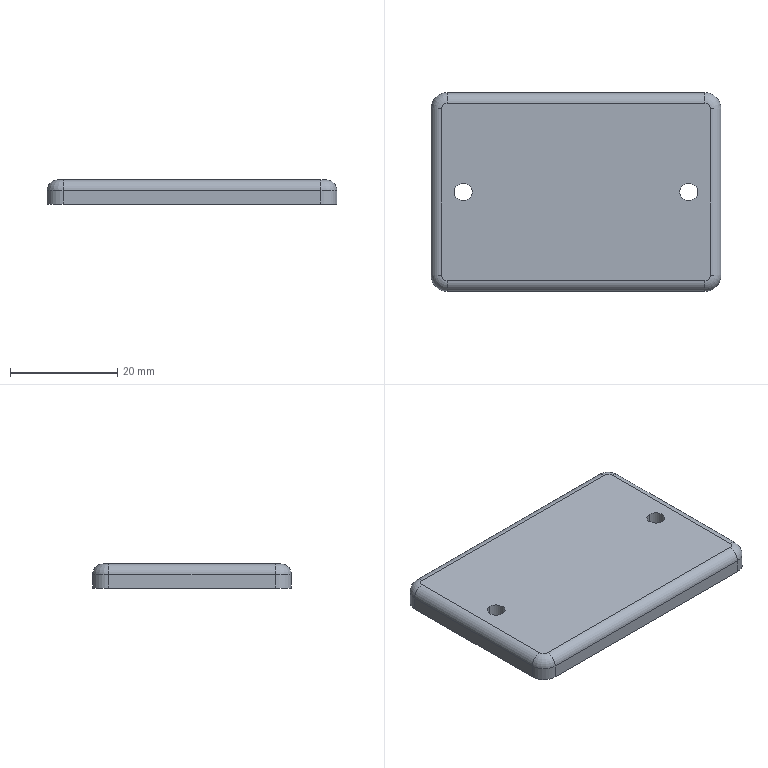Part | SolidWorks | features BaseBody 1 | 1 solid | 35 faces | box 54 x 37 x 4.5 mm | volume 8135 mm3 | cylinder 18 | plane 13 | torus 4 | commonest cylinder face diameters 11.3 x6 3.3 x4 4 x4 6 x4
STEP:
#1=CARTESIAN_POINT('',(-30.5,5.65,26.5));
#2=VERTEX_POINT('',#1);
#3=CARTESIAN_POINT('',(-30.5,5.65,26.));
#4=VERTEX_POINT('',#3);
#5=CARTESIAN_POINT('',(-30.5,5.65,31.5));
#6=DIRECTION('',(0.,0.,-1.));
#7=VECTOR('',#6,1000.);
#8=LINE('',#5,#7);
#9=EDGE_CURVE('',#2,#4,#8,.T.);
#10=ORIENTED_EDGE('',*,*,#9,.F.);
#11=CARTESIAN_POINT('',(-28.5,5.284,26.5));
#12=VERTEX_POINT('',#11);
#13=CARTESIAN_POINT('',(-30.5,0.,26.5));
#14=DIRECTION('',(0.,0.,1.));
#15=DIRECTION('',(0.,1.,0.));
#16=AXIS2_PLACEMENT_3D('',#13,#14,#15);
#17=CIRCLE('',#16,5.65);
#18=EDGE_CURVE('',#12,#2,#17,.T.);
#19=ORIENTED_EDGE('',*,*,#18,.F.);
#20=CARTESIAN_POINT('',(-28.5,5.284,26.));
#21=VERTEX_POINT('',#20);
#22=CARTESIAN_POINT('',(-28.5,5.284,31.5));
#23=DIRECTION('',(0.,0.,1.));
#24=VECTOR('',#23,1000.);
#25=LINE('',#22,#24);
#26=EDGE_CURVE('',#21,#12,#25,.T.);
#27=ORIENTED_EDGE('',*,*,#26,.F.);
#28=CARTESIAN_POINT('',(-30.5,0.,26.));
#29=DIRECTION('',(0.,0.,1.));
#30=DIRECTION('',(0.,1.,0.));
#31=AXIS2_PLACEMENT_3D('',#28,#29,#30);
#32=CIRCLE('',#31,5.65);
#33=EDGE_CURVE('',#21,#4,#32,.T.);
#34=ORIENTED_EDGE('',*,*,#33,.T.);
#35=EDGE_LOOP('',(#10,#19,#27,#34));
#36=FACE_OUTER_BOUND('',#35,.T.);
#37=CARTESIAN_POINT('',(-30.5,0.,31.5));
#38=DIRECTION('',(0.,0.,-1.));
#39=DIRECTION('',(0.,1.,0.));
#40=AXIS2_PLACEMENT_3D('',#37,#38,#39);
#41=CYLINDRICAL_SURFACE('',#40,5.65);
#42=ADVANCED_FACE('',(#36),#41,.T.);
#43=CARTESIAN_POINT('',(-72.5,-5.65,26.5));
#44=VERTEX_POINT('',#43);
#45=CARTESIAN_POINT('',(-72.5,-5.65,26.));
#46=VERTEX_POINT('',#45);
#47=CARTESIAN_POINT('',(-72.5,-5.65,31.5));
#48=DIRECTION('',(0.,0.,-1.));
#49=VECTOR('',#48,1000.);
#50=LINE('',#47,#49);
#51=EDGE_CURVE('',#44,#46,#50,.T.);
#52=ORIENTED_EDGE('',*,*,#51,.F.);
#53=CARTESIAN_POINT('',(-74.5,-5.284,26.5));
#54=VERTEX_POINT('',#53);
#55=CARTESIAN_POINT('',(-72.5,0.,26.5));
#56=DIRECTION('',(0.,0.,-1.));
#57=DIRECTION('',(0.,1.,0.));
#58=AXIS2_PLACEMENT_3D('',#55,#56,#57);
#59=CIRCLE('',#58,5.65);
#60=EDGE_CURVE('',#44,#54,#59,.T.);
#61=ORIENTED_EDGE('',*,*,#60,.T.);
#62=CARTESIAN_POINT('',(-74.5,-5.284,26.));
#63=VERTEX_POINT('',#62);
#64=CARTESIAN_POINT('',(-74.5,-5.284,31.5));
#65=DIRECTION('',(0.,0.,-1.));
#66=VECTOR('',#65,1000.);
#67=LINE('',#64,#66);
#68=EDGE_CURVE('',#54,#63,#67,.T.);
#69=ORIENTED_EDGE('',*,*,#68,.T.);
#70=CARTESIAN_POINT('',(-72.5,0.,26.));
#71=DIRECTION('',(0.,0.,-1.));
#72=DIRECTION('',(0.,1.,0.));
#73=AXIS2_PLACEMENT_3D('',#70,#71,#72);
#74=CIRCLE('',#73,5.65);
#75=EDGE_CURVE('',#46,#63,#74,.T.);
#76=ORIENTED_EDGE('',*,*,#75,.F.);
#77=EDGE_LOOP('',(#52,#61,#69,#76));
#78=FACE_OUTER_BOUND('',#77,.T.);
#79=CARTESIAN_POINT('',(-72.5,0.,31.5));
#80=DIRECTION('',(0.,0.,-1.));
#81=DIRECTION('',(0.,1.,0.));
#82=AXIS2_PLACEMENT_3D('',#79,#80,#81);
#83=CYLINDRICAL_SURFACE('',#82,5.65);
#84=ADVANCED_FACE('',(#78),#83,.T.);
#85=CARTESIAN_POINT('',(-28.5,-14.5,26.5));
#86=VERTEX_POINT('',#85);
#87=CARTESIAN_POINT('',(-28.5,-14.5,26.));
#88=VERTEX_POINT('',#87);
#89=CARTESIAN_POINT('',(-28.5,-14.5,29.5));
#90=DIRECTION('',(0.,0.,-1.));
#91=VECTOR('',#90,1000.);
#92=LINE('',#89,#91);
#93=EDGE_CURVE('',#86,#88,#92,.T.);
#94=ORIENTED_EDGE('',*,*,#93,.T.);
#95=CARTESIAN_POINT('',(-74.5,-14.5,26.));
#96=VERTEX_POINT('',#95);
#97=CARTESIAN_POINT('',(-75.5,-14.5,26.));
#98=DIRECTION('',(-1.,0.,0.));
#99=VECTOR('',#98,1000.);
#100=LINE('',#97,#99);
#101=EDGE_CURVE('',#88,#96,#100,.T.);
#102=ORIENTED_EDGE('',*,*,#101,.T.);
#103=CARTESIAN_POINT('',(-74.5,-14.5,26.5));
#104=VERTEX_POINT('',#103);
#105=CARTESIAN_POINT('',(-74.5,-14.5,29.5));
#106=DIRECTION('',(0.,0.,-1.));
#107=VECTOR('',#106,1000.);
#108=LINE('',#105,#107);
#109=EDGE_CURVE('',#104,#96,#108,.T.);
#110=ORIENTED_EDGE('',*,*,#109,.F.);
#111=CARTESIAN_POINT('',(-27.5,-14.5,26.5));
#112=DIRECTION('',(1.,0.,0.));
#113=VECTOR('',#112,1000.);
#114=LINE('',#111,#113);
#115=EDGE_CURVE('',#104,#86,#114,.T.);
#116=ORIENTED_EDGE('',*,*,#115,.T.);
#117=EDGE_LOOP('',(#94,#102,#110,#116));
#118=FACE_OUTER_BOUND('',#117,.T.);
#119=CARTESIAN_POINT('',(-27.5,-14.5,29.5));
#120=DIRECTION('',(0.,-1.,0.));
#121=DIRECTION('',(0.,0.,-1.));
#122=AXIS2_PLACEMENT_3D('',#119,#120,#121);
#123=PLANE('',#122);
#124=ADVANCED_FACE('',(#118),#123,.F.);
#125=CARTESIAN_POINT('',(-28.5,-5.284,26.));
#126=VERTEX_POINT('',#125);
#127=CARTESIAN_POINT('',(-28.5,15.5,26.));
#128=DIRECTION('',(0.,-1.,0.));
#129=VECTOR('',#128,1000.);
#130=LINE('',#127,#129);
#131=EDGE_CURVE('',#126,#88,#130,.T.);
#132=ORIENTED_EDGE('',*,*,#131,.T.);
#133=ORIENTED_EDGE('',*,*,#93,.F.);
#134=CARTESIAN_POINT('',(-28.5,-5.284,26.5));
#135=VERTEX_POINT('',#134);
#136=CARTESIAN_POINT('',(-28.5,15.5,26.5));
#137=DIRECTION('',(0.,-1.,0.));
#138=VECTOR('',#137,1000.);
#139=LINE('',#136,#138);
#140=EDGE_CURVE('',#135,#86,#139,.T.);
#141=ORIENTED_EDGE('',*,*,#140,.F.);
#142=CARTESIAN_POINT('',(-28.5,-5.284,31.5));
#143=DIRECTION('',(0.,0.,-1.));
#144=VECTOR('',#143,1000.);
#145=LINE('',#142,#144);
#146=EDGE_CURVE('',#135,#126,#145,.T.);
#147=ORIENTED_EDGE('',*,*,#146,.T.);
#148=EDGE_LOOP('',(#132,#133,#141,#147));
#149=FACE_OUTER_BOUND('',#148,.T.);
#150=CARTESIAN_POINT('',(-28.5,15.5,29.5));
#151=DIRECTION('',(1.,0.,0.));
#152=DIRECTION('',(0.,1.,0.));
#153=AXIS2_PLACEMENT_3D('',#150,#151,#152);
#154=PLANE('',#153);
#155=ADVANCED_FACE('',(#149),#154,.F.);
#156=CARTESIAN_POINT('',(-74.5,14.5,26.5));
#157=VERTEX_POINT('',#156);
#158=CARTESIAN_POINT('',(-74.5,14.5,26.));
#159=VERTEX_POINT('',#158);
#160=CARTESIAN_POINT('',(-74.5,14.5,29.5));
#161=DIRECTION('',(0.,0.,-1.));
#162=VECTOR('',#161,1000.);
#163=LINE('',#160,#162);
#164=EDGE_CURVE('',#157,#159,#163,.T.);
#165=ORIENTED_EDGE('',*,*,#164,.T.);
#166=CARTESIAN_POINT('',(-28.5,14.5,26.));
#167=VERTEX_POINT('',#166);
#168=CARTESIAN_POINT('',(-75.5,14.5,26.));
#169=DIRECTION('',(1.,0.,0.));
#170=VECTOR('',#169,1000.);
#171=LINE('',#168,#170);
#172=EDGE_CURVE('',#159,#167,#171,.T.);
#173=ORIENTED_EDGE('',*,*,#172,.T.);
#174=CARTESIAN_POINT('',(-28.5,14.5,26.5));
#175=VERTEX_POINT('',#174);
#176=CARTESIAN_POINT('',(-28.5,14.5,29.5));
#177=DIRECTION('',(0.,0.,-1.));
#178=VECTOR('',#177,1000.);
#179=LINE('',#176,#178);
#180=EDGE_CURVE('',#175,#167,#179,.T.);
#181=ORIENTED_EDGE('',*,*,#180,.F.);
#182=CARTESIAN_POINT('',(-75.5,14.5,26.5));
#183=DIRECTION('',(1.,0.,0.));
#184=VECTOR('',#183,1000.);
#185=LINE('',#182,#184);
#186=EDGE_CURVE('',#157,#175,#185,.T.);
#187=ORIENTED_EDGE('',*,*,#186,.F.);
#188=EDGE_LOOP('',(#165,#173,#181,#187));
#189=FACE_OUTER_BOUND('',#188,.T.);
#190=CARTESIAN_POINT('',(-75.5,14.5,29.5));
#191=DIRECTION('',(0.,1.,0.));
#192=DIRECTION('',(1.,0.,0.));
#193=AXIS2_PLACEMENT_3D('',#190,#191,#192);
#194=PLANE('',#193);
#195=ADVANCED_FACE('',(#189),#194,.F.);
#196=CARTESIAN_POINT('',(-74.5,5.284,26.));
#197=VERTEX_POINT('',#196);
#198=CARTESIAN_POINT('',(-74.5,5.284,26.5));
#199=VERTEX_POINT('',#198);
#200=CARTESIAN_POINT('',(-74.5,5.284,31.5));
#201=DIRECTION('',(0.,0.,1.));
#202=VECTOR('',#201,1000.);
#203=LINE('',#200,#202);
#204=EDGE_CURVE('',#197,#199,#203,.T.);
#205=ORIENTED_EDGE('',*,*,#204,.F.);
#206=CARTESIAN_POINT('',(-74.5,15.5,26.));
#207=DIRECTION('',(0.,1.,0.));
#208=VECTOR('',#207,1000.);
#209=LINE('',#206,#208);
#210=EDGE_CURVE('',#197,#159,#209,.T.);
#211=ORIENTED_EDGE('',*,*,#210,.T.);
#212=ORIENTED_EDGE('',*,*,#164,.F.);
#213=CARTESIAN_POINT('',(-74.5,-15.5,26.5));
#214=DIRECTION('',(0.,-1.,0.));
#215=VECTOR('',#214,1000.);
#216=LINE('',#213,#215);
#217=EDGE_CURVE('',#157,#199,#216,.T.);
#218=ORIENTED_EDGE('',*,*,#217,.T.);
#219=EDGE_LOOP('',(#205,#211,#212,#218));
#220=FACE_OUTER_BOUND('',#219,.T.);
#221=CARTESIAN_POINT('',(-74.5,-15.5,29.5));
#222=DIRECTION('',(-1.,0.,0.));
#223=DIRECTION('',(0.,1.,0.));
#224=AXIS2_PLACEMENT_3D('',#221,#222,#223);
#225=PLANE('',#224);
#226=ADVANCED_FACE('',(#220),#225,.F.);
#227=ORIENTED_EDGE('',*,*,#140,.T.);
#228=ORIENTED_EDGE('',*,*,#115,.F.);
#229=CARTESIAN_POINT('',(-74.5,-15.5,26.5));
#230=DIRECTION('',(0.,-1.,0.));
#231=VECTOR('',#230,1000.);
#232=LINE('',#229,#231);
#233=EDGE_CURVE('',#54,#104,#232,.T.);
#234=ORIENTED_EDGE('',*,*,#233,.F.);
#235=ORIENTED_EDGE('',*,*,#60,.F.);
#236=CARTESIAN_POINT('',(-72.5,5.65,26.5));
#237=VERTEX_POINT('',#236);
#238=CARTESIAN_POINT('',(-72.5,0.,26.5));
#239=DIRECTION('',(0.,0.,-1.));
#240=DIRECTION('',(0.,1.,0.));
#241=AXIS2_PLACEMENT_3D('',#238,#239,#240);
#242=CIRCLE('',#241,5.65);
#243=EDGE_CURVE('',#237,#44,#242,.T.);
#244=ORIENTED_EDGE('',*,*,#243,.F.);
#245=CARTESIAN_POINT('',(-72.5,0.,26.5));
#246=DIRECTION('',(0.,0.,-1.));
#247=DIRECTION('',(0.,1.,0.));
#248=AXIS2_PLACEMENT_3D('',#245,#246,#247);
#249=CIRCLE('',#248,5.65);
#250=EDGE_CURVE('',#199,#237,#249,.T.);
#251=ORIENTED_EDGE('',*,*,#250,.F.);
#252=ORIENTED_EDGE('',*,*,#217,.F.);
#253=ORIENTED_EDGE('',*,*,#186,.T.);
#254=CARTESIAN_POINT('',(-28.5,15.5,26.5));
#255=DIRECTION('',(0.,-1.,0.));
#256=VECTOR('',#255,1000.);
#257=LINE('',#254,#256);
#258=EDGE_CURVE('',#175,#12,#257,.T.);
#259=ORIENTED_EDGE('',*,*,#258,.T.);
#260=ORIENTED_EDGE('',*,*,#18,.T.);
#261=CARTESIAN_POINT('',(-30.5,-5.65,26.5));
#262=VERTEX_POINT('',#261);
#263=CARTESIAN_POINT('',(-30.5,0.,26.5));
#264=DIRECTION('',(0.,0.,1.));
#265=DIRECTION('',(0.,1.,0.));
#266=AXIS2_PLACEMENT_3D('',#263,#264,#265);
#267=CIRCLE('',#266,5.65);
#268=EDGE_CURVE('',#2,#262,#267,.T.);
#269=ORIENTED_EDGE('',*,*,#268,.T.);
#270=CARTESIAN_POINT('',(-30.5,0.,26.5));
#271=DIRECTION('',(0.,0.,1.));
#272=DIRECTION('',(0.,1.,0.));
#273=AXIS2_PLACEMENT_3D('',#270,#271,#272);
#274=CIRCLE('',#273,5.65);
#275=EDGE_CURVE('',#262,#135,#274,.T.);
#276=ORIENTED_EDGE('',*,*,#275,.T.);
#277=EDGE_LOOP('',(#227,#228,#234,#235,#244,#251,#252,#253,#259,#260,#269,#276));
#278=FACE_OUTER_BOUND('',#277,.T.);
#279=CARTESIAN_POINT('',(-75.5,15.5,26.5));
#280=DIRECTION('',(0.,0.,-1.));
#281=DIRECTION('',(0.,-1.,0.));
#282=AXIS2_PLACEMENT_3D('',#279,#280,#281);
#283=PLANE('',#282);
#284=ADVANCED_FACE('',(#278),#283,.T.);
#285=ORIENTED_EDGE('',*,*,#26,.T.);
#286=ORIENTED_EDGE('',*,*,#258,.F.);
#287=ORIENTED_EDGE('',*,*,#180,.T.);
#288=CARTESIAN_POINT('',(-28.5,15.5,26.));
#289=DIRECTION('',(0.,-1.,0.));
#290=VECTOR('',#289,1000.);
#291=LINE('',#288,#290);
#292=EDGE_CURVE('',#167,#21,#291,.T.);
#293=ORIENTED_EDGE('',*,*,#292,.T.);
#294=EDGE_LOOP('',(#285,#286,#287,#293));
#295=FACE_OUTER_BOUND('',#294,.T.);
#296=CARTESIAN_POINT('',(-28.5,15.5,29.5));
#297=DIRECTION('',(1.,0.,0.));
#298=DIRECTION('',(0.,1.,0.));
#299=AXIS2_PLACEMENT_3D('',#296,#297,#298);
#300=PLANE('',#299);
#301=ADVANCED_FACE('',(#295),#300,.F.);
#302=ORIENTED_EDGE('',*,*,#233,.T.);
#303=ORIENTED_EDGE('',*,*,#109,.T.);
#304=CARTESIAN_POINT('',(-74.5,15.5,26.));
#305=DIRECTION('',(0.,1.,0.));
#306=VECTOR('',#305,1000.);
#307=LINE('',#304,#306);
#308=EDGE_CURVE('',#96,#63,#307,.T.);
#309=ORIENTED_EDGE('',*,*,#308,.T.);
#310=ORIENTED_EDGE('',*,*,#68,.F.);
#311=EDGE_LOOP('',(#302,#303,#309,#310));
#312=FACE_OUTER_BOUND('',#311,.T.);
#313=CARTESIAN_POINT('',(-74.5,-15.5,29.5));
#314=DIRECTION('',(-1.,0.,0.));
#315=DIRECTION('',(0.,1.,0.));
#316=AXIS2_PLACEMENT_3D('',#313,#314,#315);
#317=PLANE('',#316);
#318=ADVANCED_FACE('',(#312),#317,.F.);
#319=CARTESIAN_POINT('',(-78.5,15.5,28.5));
#320=VERTEX_POINT('',#319);
#321=CARTESIAN_POINT('',(-76.5,15.5,30.5));
#322=VERTEX_POINT('',#321);
#323=CARTESIAN_POINT('',(-76.5,15.5,28.5));
#324=DIRECTION('',(0.,1.,0.));
#325=DIRECTION('',(0.,0.,1.));
#326=AXIS2_PLACEMENT_3D('',#323,#324,#325);
#327=CIRCLE('',#326,2.);
#328=EDGE_CURVE('',#320,#322,#327,.T.);
#329=ORIENTED_EDGE('',*,*,#328,.T.);
#330=CARTESIAN_POINT('',(-75.5,16.5,30.5));
#331=VERTEX_POINT('',#330);
#332=CARTESIAN_POINT('',(-75.5,15.5,30.5));
#333=DIRECTION('',(0.,0.,1.));
#334=DIRECTION('',(0.,1.,0.));
#335=AXIS2_PLACEMENT_3D('',#332,#333,#334);
#336=CIRCLE('',#335,1.);
#337=EDGE_CURVE('',#331,#322,#336,.T.);
#338=ORIENTED_EDGE('',*,*,#337,.F.);
#339=CARTESIAN_POINT('',(-75.5,18.5,28.5));
#340=VERTEX_POINT('',#339);
#341=CARTESIAN_POINT('',(-75.5,16.5,28.5));
#342=DIRECTION('',(-1.,0.,0.));
#343=DIRECTION('',(0.,0.,-1.));
#344=AXIS2_PLACEMENT_3D('',#341,#342,#343);
#345=CIRCLE('',#344,2.);
#346=EDGE_CURVE('',#331,#340,#345,.T.);
#347=ORIENTED_EDGE('',*,*,#346,.T.);
#348=CARTESIAN_POINT('',(-75.5,15.5,28.5));
#349=DIRECTION('',(0.,0.,-1.));
#350=DIRECTION('',(0.,1.,0.));
#351=AXIS2_PLACEMENT_3D('',#348,#349,#350);
#352=CIRCLE('',#351,3.);
#353=EDGE_CURVE('',#320,#340,#352,.T.);
#354=ORIENTED_EDGE('',*,*,#353,.F.);
#355=EDGE_LOOP('',(#329,#338,#347,#354));
#356=FACE_OUTER_BOUND('',#355,.T.);
#357=CARTESIAN_POINT('',(-75.5,15.5,28.5));
#358=DIRECTION('',(0.,0.,-1.));
#359=DIRECTION('',(0.,1.,0.));
#360=AXIS2_PLACEMENT_3D('',#357,#358,#359);
#361=TOROIDAL_SURFACE('',#360,1.,2.);
#362=ADVANCED_FACE('',(#356),#361,.T.);
#363=CARTESIAN_POINT('',(-27.5,16.5,30.5));
#364=VERTEX_POINT('',#363);
#365=CARTESIAN_POINT('',(-27.5,18.5,28.5));
#366=VERTEX_POINT('',#365);
#367=CARTESIAN_POINT('',(-27.5,16.5,28.5));
#368=DIRECTION('',(-1.,0.,0.));
#369=DIRECTION('',(0.,1.,0.));
#370=AXIS2_PLACEMENT_3D('',#367,#368,#369);
#371=CIRCLE('',#370,2.);
#372=EDGE_CURVE('',#364,#366,#371,.T.);
#373=ORIENTED_EDGE('',*,*,#372,.T.);
#374=CARTESIAN_POINT('',(-27.5,18.5,28.5));
#375=DIRECTION('',(1.,0.,0.));
#376=VECTOR('',#375,1000.);
#377=LINE('',#374,#376);
#378=EDGE_CURVE('',#340,#366,#377,.T.);
#379=ORIENTED_EDGE('',*,*,#378,.F.);
#380=ORIENTED_EDGE('',*,*,#346,.F.);
#381=CARTESIAN_POINT('',(-75.5,16.5,30.5));
#382=DIRECTION('',(-1.,0.,0.));
#383=VECTOR('',#382,1000.);
#384=LINE('',#381,#383);
#385=EDGE_CURVE('',#364,#331,#384,.T.);
#386=ORIENTED_EDGE('',*,*,#385,.F.);
#387=EDGE_LOOP('',(#373,#379,#380,#386));
#388=FACE_OUTER_BOUND('',#387,.T.);
#389=CARTESIAN_POINT('',(-75.5,16.5,28.5));
#390=DIRECTION('',(-1.,0.,0.));
#391=DIRECTION('',(0.,0.,-1.));
#392=AXIS2_PLACEMENT_3D('',#389,#390,#391);
#393=CYLINDRICAL_SURFACE('',#392,2.);
#394=ADVANCED_FACE('',(#388),#393,.T.);
#395=CARTESIAN_POINT('',(-78.5,-15.5,28.5));
#396=VERTEX_POINT('',#395);
#397=CARTESIAN_POINT('',(-76.5,-15.5,30.5));
#398=VERTEX_POINT('',#397);
#399=CARTESIAN_POINT('',(-76.5,-15.5,28.5));
#400=DIRECTION('',(0.,1.,0.));
#401=DIRECTION('',(0.,0.,-1.));
#402=AXIS2_PLACEMENT_3D('',#399,#400,#401);
#403=CIRCLE('',#402,2.);
#404=EDGE_CURVE('',#396,#398,#403,.T.);
#405=ORIENTED_EDGE('',*,*,#404,.T.);
#406=CARTESIAN_POINT('',(-76.5,-15.5,30.5));
#407=DIRECTION('',(0.,-1.,0.));
#408=VECTOR('',#407,1000.);
#409=LINE('',#406,#408);
#410=EDGE_CURVE('',#322,#398,#409,.T.);
#411=ORIENTED_EDGE('',*,*,#410,.F.);
#412=ORIENTED_EDGE('',*,*,#328,.F.);
#413=CARTESIAN_POINT('',(-78.5,15.5,28.5));
#414=DIRECTION('',(0.,1.,0.));
#415=VECTOR('',#414,1000.);
#416=LINE('',#413,#415);
#417=EDGE_CURVE('',#396,#320,#416,.T.);
#418=ORIENTED_EDGE('',*,*,#417,.F.);
#419=EDGE_LOOP('',(#405,#411,#412,#418));
#420=FACE_OUTER_BOUND('',#419,.T.);
#421=CARTESIAN_POINT('',(-76.5,-15.5,28.5));
#422=DIRECTION('',(0.,-1.,0.));
#423=DIRECTION('',(0.,0.,-1.));
#424=AXIS2_PLACEMENT_3D('',#421,#422,#423);
#425=CYLINDRICAL_SURFACE('',#424,2.);
#426=ADVANCED_FACE('',(#420),#425,.T.);
#427=CARTESIAN_POINT('',(-26.5,15.5,30.5));
#428=VERTEX_POINT('',#427);
#429=CARTESIAN_POINT('',(-24.5,15.5,28.5));
#430=VERTEX_POINT('',#429);
#431=CARTESIAN_POINT('',(-26.5,15.5,28.5));
#432=DIRECTION('',(0.,1.,0.));
#433=DIRECTION('',(-1.,0.,0.));
#434=AXIS2_PLACEMENT_3D('',#431,#432,#433);
#435=CIRCLE('',#434,2.);
#436=EDGE_CURVE('',#428,#430,#435,.T.);
#437=ORIENTED_EDGE('',*,*,#436,.T.);
#438=CARTESIAN_POINT('',(-27.5,15.5,28.5));
#439=DIRECTION('',(0.,0.,-1.));
#440=DIRECTION('',(0.,1.,0.));
#441=AXIS2_PLACEMENT_3D('',#438,#439,#440);
#442=CIRCLE('',#441,3.);
#443=EDGE_CURVE('',#366,#430,#442,.T.);
#444=ORIENTED_EDGE('',*,*,#443,.F.);
#445=ORIENTED_EDGE('',*,*,#372,.F.);
#446=CARTESIAN_POINT('',(-27.5,15.5,30.5));
#447=DIRECTION('',(0.,0.,1.));
#448=DIRECTION('',(0.,1.,0.));
#449=AXIS2_PLACEMENT_3D('',#446,#447,#448);
#450=CIRCLE('',#449,1.);
#451=EDGE_CURVE('',#428,#364,#450,.T.);
#452=ORIENTED_EDGE('',*,*,#451,.F.);
#453=EDGE_LOOP('',(#437,#444,#445,#452));
#454=FACE_OUTER_BOUND('',#453,.T.);
#455=CARTESIAN_POINT('',(-27.5,15.5,28.5));
#456=DIRECTION('',(0.,0.,-1.));
#457=DIRECTION('',(0.,1.,0.));
#458=AXIS2_PLACEMENT_3D('',#455,#456,#457);
#459=TOROIDAL_SURFACE('',#458,1.,2.);
#460=ADVANCED_FACE('',(#454),#459,.T.);
#461=CARTESIAN_POINT('',(-75.5,-18.5,28.5));
#462=VERTEX_POINT('',#461);
#463=CARTESIAN_POINT('',(-75.5,-16.5,30.5));
#464=VERTEX_POINT('',#463);
#465=CARTESIAN_POINT('',(-75.5,-16.5,28.5));
#466=DIRECTION('',(-1.,0.,0.));
#467=DIRECTION('',(0.,0.,-1.));
#468=AXIS2_PLACEMENT_3D('',#465,#466,#467);
#469=CIRCLE('',#468,2.);
#470=EDGE_CURVE('',#462,#464,#469,.T.);
#471=ORIENTED_EDGE('',*,*,#470,.T.);
#472=CARTESIAN_POINT('',(-75.5,-15.5,30.5));
#473=DIRECTION('',(0.,0.,1.));
#474=DIRECTION('',(0.,1.,0.));
#475=AXIS2_PLACEMENT_3D('',#472,#473,#474);
#476=CIRCLE('',#475,1.);
#477=EDGE_CURVE('',#398,#464,#476,.T.);
#478=ORIENTED_EDGE('',*,*,#477,.F.);
#479=ORIENTED_EDGE('',*,*,#404,.F.);
#480=CARTESIAN_POINT('',(-75.5,-15.5,28.5));
#481=DIRECTION('',(0.,0.,-1.));
#482=DIRECTION('',(0.,1.,0.));
#483=AXIS2_PLACEMENT_3D('',#480,#481,#482);
#484=CIRCLE('',#483,3.);
#485=EDGE_CURVE('',#462,#396,#484,.T.);
#486=ORIENTED_EDGE('',*,*,#485,.F.);
#487=EDGE_LOOP('',(#471,#478,#479,#486));
#488=FACE_OUTER_BOUND('',#487,.T.);
#489=CARTESIAN_POINT('',(-75.5,-15.5,28.5));
#490=DIRECTION('',(0.,0.,-1.));
#491=DIRECTION('',(0.,1.,0.));
#492=AXIS2_PLACEMENT_3D('',#489,#490,#491);
#493=TOROIDAL_SURFACE('',#492,1.,2.);
#494=ADVANCED_FACE('',(#488),#493,.T.);
#495=CARTESIAN_POINT('',(-26.5,-15.5,30.5));
#496=VERTEX_POINT('',#495);
#497=CARTESIAN_POINT('',(-24.5,-15.5,28.5));
#498=VERTEX_POINT('',#497);
#499=CARTESIAN_POINT('',(-26.5,-15.5,28.5));
#500=DIRECTION('',(0.,1.,0.));
#501=DIRECTION('',(1.,0.,0.));
#502=AXIS2_PLACEMENT_3D('',#499,#500,#501);
#503=CIRCLE('',#502,2.);
#504=EDGE_CURVE('',#496,#498,#503,.T.);
#505=ORIENTED_EDGE('',*,*,#504,.T.);
#506=CARTESIAN_POINT('',(-24.5,-15.5,28.5));
#507=DIRECTION('',(0.,-1.,0.));
#508=VECTOR('',#507,1000.);
#509=LINE('',#506,#508);
#510=EDGE_CURVE('',#430,#498,#509,.T.);
#511=ORIENTED_EDGE('',*,*,#510,.F.);
#512=ORIENTED_EDGE('',*,*,#436,.F.);
#513=CARTESIAN_POINT('',(-26.5,15.5,30.5));
#514=DIRECTION('',(0.,1.,0.));
#515=VECTOR('',#514,1000.);
#516=LINE('',#513,#515);
#517=EDGE_CURVE('',#496,#428,#516,.T.);
#518=ORIENTED_EDGE('',*,*,#517,.F.);
#519=EDGE_LOOP('',(#505,#511,#512,#518));
#520=FACE_OUTER_BOUND('',#519,.T.);
#521=CARTESIAN_POINT('',(-26.5,15.5,28.5));
#522=DIRECTION('',(0.,1.,0.));
#523=DIRECTION('',(-1.,0.,0.));
#524=AXIS2_PLACEMENT_3D('',#521,#522,#523);
#525=CYLINDRICAL_SURFACE('',#524,2.);
#526=ADVANCED_FACE('',(#520),#525,.T.);
#527=CARTESIAN_POINT('',(-27.5,-18.5,28.5));
#528=VERTEX_POINT('',#527);
#529=CARTESIAN_POINT('',(-27.5,-16.5,30.5));
#530=VERTEX_POINT('',#529);
#531=CARTESIAN_POINT('',(-27.5,-16.5,28.5));
#532=DIRECTION('',(-1.,0.,0.));
#533=DIRECTION('',(0.,0.,1.));
#534=AXIS2_PLACEMENT_3D('',#531,#532,#533);
#535=CIRCLE('',#534,2.);
#536=EDGE_CURVE('',#528,#530,#535,.T.);
#537=ORIENTED_EDGE('',*,*,#536,.T.);
#538=CARTESIAN_POINT('',(-27.5,-16.5,30.5));
#539=DIRECTION('',(1.,0.,0.));
#540=VECTOR('',#539,1000.);
#541=LINE('',#538,#540);
#542=EDGE_CURVE('',#464,#530,#541,.T.);
#543=ORIENTED_EDGE('',*,*,#542,.F.);
#544=ORIENTED_EDGE('',*,*,#470,.F.);
#545=CARTESIAN_POINT('',(-75.5,-18.5,28.5));
#546=DIRECTION('',(-1.,0.,0.));
#547=VECTOR('',#546,1000.);
#548=LINE('',#545,#547);
#549=EDGE_CURVE('',#528,#462,#548,.T.);
#550=ORIENTED_EDGE('',*,*,#549,.F.);
#551=EDGE_LOOP('',(#537,#543,#544,#550));
#552=FACE_OUTER_BOUND('',#551,.T.);
#553=CARTESIAN_POINT('',(-27.5,-16.5,28.5));
#554=DIRECTION('',(1.,0.,0.));
#555=DIRECTION('',(0.,0.,1.));
#556=AXIS2_PLACEMENT_3D('',#553,#554,#555);
#557=CYLINDRICAL_SURFACE('',#556,2.);
#558=ADVANCED_FACE('',(#552),#557,.T.);
#559=ORIENTED_EDGE('',*,*,#504,.F.);
#560=CARTESIAN_POINT('',(-27.5,-15.5,30.5));
#561=DIRECTION('',(0.,0.,1.));
#562=DIRECTION('',(0.,1.,0.));
#563=AXIS2_PLACEMENT_3D('',#560,#561,#562);
#564=CIRCLE('',#563,1.);
#565=EDGE_CURVE('',#530,#496,#564,.T.);
#566=ORIENTED_EDGE('',*,*,#565,.F.);
#567=ORIENTED_EDGE('',*,*,#536,.F.);
#568=CARTESIAN_POINT('',(-27.5,-15.5,28.5));
#569=DIRECTION('',(0.,0.,-1.));
#570=DIRECTION('',(0.,1.,0.));
#571=AXIS2_PLACEMENT_3D('',#568,#569,#570);
#572=CIRCLE('',#571,3.);
#573=EDGE_CURVE('',#498,#528,#572,.T.);
#574=ORIENTED_EDGE('',*,*,#573,.F.);
#575=EDGE_LOOP('',(#559,#566,#567,#574));
#576=FACE_OUTER_BOUND('',#575,.T.);
#577=CARTESIAN_POINT('',(-27.5,-15.5,28.5));
#578=DIRECTION('',(0.,0.,-1.));
#579=DIRECTION('',(0.,1.,0.));
#580=AXIS2_PLACEMENT_3D('',#577,#578,#579);
#581=TOROIDAL_SURFACE('',#580,1.,2.);
#582=ADVANCED_FACE('',(#576),#581,.T.);
#583=CARTESIAN_POINT('',(-30.5,-1.65,30.5));
#584=VERTEX_POINT('',#583);
#585=CARTESIAN_POINT('',(-30.5,-1.65,26.));
#586=VERTEX_POINT('',#585);
#587=CARTESIAN_POINT('',(-30.5,-1.65,31.5));
#588=DIRECTION('',(0.,0.,-1.));
#589=VECTOR('',#588,1000.);
#590=LINE('',#587,#589);
#591=EDGE_CURVE('',#584,#586,#590,.T.);
#592=ORIENTED_EDGE('',*,*,#591,.F.);
#593=CARTESIAN_POINT('',(-30.5,1.65,30.5));
#594=VERTEX_POINT('',#593);
#595=CARTESIAN_POINT('',(-30.5,0.,30.5));
#596=DIRECTION('',(0.,0.,1.));
#597=DIRECTION('',(0.,1.,0.));
#598=AXIS2_PLACEMENT_3D('',#595,#596,#597);
#599=CIRCLE('',#598,1.65);
#600=EDGE_CURVE('',#584,#594,#599,.T.);
#601=ORIENTED_EDGE('',*,*,#600,.T.);
#602=CARTESIAN_POINT('',(-30.5,1.65,26.));
#603=VERTEX_POINT('',#602);
#604=CARTESIAN_POINT('',(-30.5,1.65,31.5));
#605=DIRECTION('',(0.,0.,-1.));
#606=VECTOR('',#605,1000.);
#607=LINE('',#604,#606);
#608=EDGE_CURVE('',#594,#603,#607,.T.);
#609=ORIENTED_EDGE('',*,*,#608,.T.);
#610=CARTESIAN_POINT('',(-30.5,0.,26.));
#611=DIRECTION('',(0.,0.,1.));
#612=DIRECTION('',(0.,1.,0.));
#613=AXIS2_PLACEMENT_3D('',#610,#611,#612);
#614=CIRCLE('',#613,1.65);
#615=EDGE_CURVE('',#586,#603,#614,.T.);
#616=ORIENTED_EDGE('',*,*,#615,.F.);
#617=EDGE_LOOP('',(#592,#601,#609,#616));
#618=FACE_OUTER_BOUND('',#617,.T.);
#619=CARTESIAN_POINT('',(-30.5,0.,31.5));
#620=DIRECTION('',(0.,0.,-1.));
#621=DIRECTION('',(0.,1.,0.));
#622=AXIS2_PLACEMENT_3D('',#619,#620,#621);
#623=CYLINDRICAL_SURFACE('',#622,1.65);
#624=ADVANCED_FACE('',(#618),#623,.F.);
#625=CARTESIAN_POINT('',(-72.5,-1.65,30.5));
#626=VERTEX_POINT('',#625);
#627=CARTESIAN_POINT('',(-72.5,-1.65,26.));
#628=VERTEX_POINT('',#627);
#629=CARTESIAN_POINT('',(-72.5,-1.65,31.5));
#630=DIRECTION('',(0.,0.,-1.));
#631=VECTOR('',#630,1000.);
#632=LINE('',#629,#631);
#633=EDGE_CURVE('',#626,#628,#632,.T.);
#634=ORIENTED_EDGE('',*,*,#633,.F.);
#635=CARTESIAN_POINT('',(-72.5,1.65,30.5));
#636=VERTEX_POINT('',#635);
#637=CARTESIAN_POINT('',(-72.5,0.,30.5));
#638=DIRECTION('',(0.,0.,-1.));
#639=DIRECTION('',(0.,1.,0.));
#640=AXIS2_PLACEMENT_3D('',#637,#638,#639);
#641=CIRCLE('',#640,1.65);
#642=EDGE_CURVE('',#636,#626,#641,.T.);
#643=ORIENTED_EDGE('',*,*,#642,.F.);
#644=CARTESIAN_POINT('',(-72.5,1.65,26.));
#645=VERTEX_POINT('',#644);
#646=CARTESIAN_POINT('',(-72.5,1.65,31.5));
#647=DIRECTION('',(0.,0.,-1.));
#648=VECTOR('',#647,1000.);
#649=LINE('',#646,#648);
#650=EDGE_CURVE('',#636,#645,#649,.T.);
#651=ORIENTED_EDGE('',*,*,#650,.T.);
#652=CARTESIAN_POINT('',(-72.5,0.,26.));
#653=DIRECTION('',(0.,0.,-1.));
#654=DIRECTION('',(0.,1.,0.));
#655=AXIS2_PLACEMENT_3D('',#652,#653,#654);
#656=CIRCLE('',#655,1.65);
#657=EDGE_CURVE('',#645,#628,#656,.T.);
#658=ORIENTED_EDGE('',*,*,#657,.T.);
#659=EDGE_LOOP('',(#634,#643,#651,#658));
#660=FACE_OUTER_BOUND('',#659,.T.);
#661=CARTESIAN_POINT('',(-72.5,0.,31.5));
#662=DIRECTION('',(0.,0.,-1.));
#663=DIRECTION('',(0.,1.,0.));
#664=AXIS2_PLACEMENT_3D('',#661,#662,#663);
#665=CYLINDRICAL_SURFACE('',#664,1.65);
#666=ADVANCED_FACE('',(#660),#665,.F.);
#667=CARTESIAN_POINT('',(-75.5,-18.5,26.));
#668=VERTEX_POINT('',#667);
#669=CARTESIAN_POINT('',(-75.5,-18.5,29.5));
#670=DIRECTION('',(0.,0.,-1.));
#671=VECTOR('',#670,1000.);
#672=LINE('',#669,#671);
#673=EDGE_CURVE('',#462,#668,#672,.T.);
#674=ORIENTED_EDGE('',*,*,#673,.F.);
#675=ORIENTED_EDGE('',*,*,#485,.T.);
#676=CARTESIAN_POINT('',(-78.5,-15.5,26.));
#677=VERTEX_POINT('',#676);
#678=CARTESIAN_POINT('',(-78.5,-15.5,29.5));
#679=DIRECTION('',(0.,0.,-1.));
#680=VECTOR('',#679,1000.);
#681=LINE('',#678,#680);
#682=EDGE_CURVE('',#396,#677,#681,.T.);
#683=ORIENTED_EDGE('',*,*,#682,.T.);
#684=CARTESIAN_POINT('',(-75.5,-15.5,26.));
#685=DIRECTION('',(0.,0.,-1.));
#686=DIRECTION('',(0.,-1.,0.));
#687=AXIS2_PLACEMENT_3D('',#684,#685,#686);
#688=CIRCLE('',#687,3.);
#689=EDGE_CURVE('',#668,#677,#688,.T.);
#690=ORIENTED_EDGE('',*,*,#689,.F.);
#691=EDGE_LOOP('',(#674,#675,#683,#690));
#692=FACE_OUTER_BOUND('',#691,.T.);
#693=CARTESIAN_POINT('',(-75.5,-15.5,29.5));
#694=DIRECTION('',(0.,0.,-1.));
#695=DIRECTION('',(0.,1.,0.));
#696=AXIS2_PLACEMENT_3D('',#693,#694,#695);
#697=CYLINDRICAL_SURFACE('',#696,3.);
#698=ADVANCED_FACE('',(#692),#697,.T.);
#699=CARTESIAN_POINT('',(-27.5,-18.5,26.));
#700=VERTEX_POINT('',#699);
#701=CARTESIAN_POINT('',(-27.5,-18.5,29.5));
#702=DIRECTION('',(0.,0.,-1.));
#703=VECTOR('',#702,1000.);
#704=LINE('',#701,#703);
#705=EDGE_CURVE('',#528,#700,#704,.T.);
#706=ORIENTED_EDGE('',*,*,#705,.F.);
#707=ORIENTED_EDGE('',*,*,#549,.T.);
#708=ORIENTED_EDGE('',*,*,#673,.T.);
#709=CARTESIAN_POINT('',(-27.5,-18.5,26.));
#710=DIRECTION('',(-1.,0.,0.));
#711=VECTOR('',#710,1000.);
#712=LINE('',#709,#711);
#713=EDGE_CURVE('',#700,#668,#712,.T.);
#714=ORIENTED_EDGE('',*,*,#713,.F.);
#715=EDGE_LOOP('',(#706,#707,#708,#714));
#716=FACE_OUTER_BOUND('',#715,.T.);
#717=CARTESIAN_POINT('',(-27.5,-18.5,29.5));
#718=DIRECTION('',(0.,-1.,0.));
#719=DIRECTION('',(0.,0.,-1.));
#720=AXIS2_PLACEMENT_3D('',#717,#718,#719);
#721=PLANE('',#720);
#722=ADVANCED_FACE('',(#716),#721,.T.);
#723=CARTESIAN_POINT('',(-24.5,-15.5,26.));
#724=VERTEX_POINT('',#723);
#725=CARTESIAN_POINT('',(-24.5,-15.5,29.5));
#726=DIRECTION('',(0.,0.,-1.));
#727=VECTOR('',#726,1000.);
#728=LINE('',#725,#727);
#729=EDGE_CURVE('',#498,#724,#728,.T.);
#730=ORIENTED_EDGE('',*,*,#729,.F.);
#731=ORIENTED_EDGE('',*,*,#573,.T.);
#732=ORIENTED_EDGE('',*,*,#705,.T.);
#733=CARTESIAN_POINT('',(-27.5,-15.5,26.));
#734=DIRECTION('',(0.,0.,-1.));
#735=DIRECTION('',(0.,-1.,0.));
#736=AXIS2_PLACEMENT_3D('',#733,#734,#735);
#737=CIRCLE('',#736,3.);
#738=EDGE_CURVE('',#724,#700,#737,.T.);
#739=ORIENTED_EDGE('',*,*,#738,.F.);
#740=EDGE_LOOP('',(#730,#731,#732,#739));
#741=FACE_OUTER_BOUND('',#740,.T.);
#742=CARTESIAN_POINT('',(-27.5,-15.5,29.5));
#743=DIRECTION('',(0.,0.,-1.));
#744=DIRECTION('',(0.,1.,0.));
#745=AXIS2_PLACEMENT_3D('',#742,#743,#744);
#746=CYLINDRICAL_SURFACE('',#745,3.);
#747=ADVANCED_FACE('',(#741),#746,.T.);
#748=CARTESIAN_POINT('',(-24.5,15.5,26.));
#749=VERTEX_POINT('',#748);
#750=CARTESIAN_POINT('',(-24.5,15.5,29.5));
#751=DIRECTION('',(0.,0.,-1.));
#752=VECTOR('',#751,1000.);
#753=LINE('',#750,#752);
#754=EDGE_CURVE('',#430,#749,#753,.T.);
#755=ORIENTED_EDGE('',*,*,#754,.F.);
#756=ORIENTED_EDGE('',*,*,#510,.T.);
#757=ORIENTED_EDGE('',*,*,#729,.T.);
#758=CARTESIAN_POINT('',(-24.5,15.5,26.));
#759=DIRECTION('',(0.,-1.,0.));
#760=VECTOR('',#759,1000.);
#761=LINE('',#758,#760);
#762=EDGE_CURVE('',#749,#724,#761,.T.);
#763=ORIENTED_EDGE('',*,*,#762,.F.);
#764=EDGE_LOOP('',(#755,#756,#757,#763));
#765=FACE_OUTER_BOUND('',#764,.T.);
#766=CARTESIAN_POINT('',(-24.5,15.5,29.5));
#767=DIRECTION('',(1.,0.,0.));
#768=DIRECTION('',(0.,1.,0.));
#769=AXIS2_PLACEMENT_3D('',#766,#767,#768);
#770=PLANE('',#769);
#771=ADVANCED_FACE('',(#765),#770,.T.);
#772=CARTESIAN_POINT('',(-27.5,18.5,26.));
#773=VERTEX_POINT('',#772);
#774=CARTESIAN_POINT('',(-27.5,18.5,29.5));
#775=DIRECTION('',(0.,0.,-1.));
#776=VECTOR('',#775,1000.);
#777=LINE('',#774,#776);
#778=EDGE_CURVE('',#366,#773,#777,.T.);
#779=ORIENTED_EDGE('',*,*,#778,.F.);
#780=ORIENTED_EDGE('',*,*,#443,.T.);
#781=ORIENTED_EDGE('',*,*,#754,.T.);
#782=CARTESIAN_POINT('',(-27.5,15.5,26.));
#783=DIRECTION('',(0.,0.,-1.));
#784=DIRECTION('',(0.,-1.,0.));
#785=AXIS2_PLACEMENT_3D('',#782,#783,#784);
#786=CIRCLE('',#785,3.);
#787=EDGE_CURVE('',#773,#749,#786,.T.);
#788=ORIENTED_EDGE('',*,*,#787,.F.);
#789=EDGE_LOOP('',(#779,#780,#781,#788));
#790=FACE_OUTER_BOUND('',#789,.T.);
#791=CARTESIAN_POINT('',(-27.5,15.5,29.5));
#792=DIRECTION('',(0.,0.,-1.));
#793=DIRECTION('',(0.,1.,0.));
#794=AXIS2_PLACEMENT_3D('',#791,#792,#793);
#795=CYLINDRICAL_SURFACE('',#794,3.);
#796=ADVANCED_FACE('',(#790),#795,.T.);
#797=CARTESIAN_POINT('',(-75.5,18.5,26.));
#798=VERTEX_POINT('',#797);
#799=CARTESIAN_POINT('',(-75.5,18.5,29.5));
#800=DIRECTION('',(0.,0.,-1.));
#801=VECTOR('',#800,1000.);
#802=LINE('',#799,#801);
#803=EDGE_CURVE('',#340,#798,#802,.T.);
#804=ORIENTED_EDGE('',*,*,#803,.F.);
#805=ORIENTED_EDGE('',*,*,#378,.T.);
#806=ORIENTED_EDGE('',*,*,#778,.T.);
#807=CARTESIAN_POINT('',(-75.5,18.5,26.));
#808=DIRECTION('',(1.,0.,0.));
#809=VECTOR('',#808,1000.);
#810=LINE('',#807,#809);
#811=EDGE_CURVE('',#798,#773,#810,.T.);
#812=ORIENTED_EDGE('',*,*,#811,.F.);
#813=EDGE_LOOP('',(#804,#805,#806,#812));
#814=FACE_OUTER_BOUND('',#813,.T.);
#815=CARTESIAN_POINT('',(-75.5,18.5,29.5));
#816=DIRECTION('',(0.,1.,0.));
#817=DIRECTION('',(1.,0.,0.));
#818=AXIS2_PLACEMENT_3D('',#815,#816,#817);
#819=PLANE('',#818);
#820=ADVANCED_FACE('',(#814),#819,.T.);
#821=CARTESIAN_POINT('',(-78.5,15.5,26.));
#822=VERTEX_POINT('',#821);
#823=CARTESIAN_POINT('',(-78.5,15.5,29.5));
#824=DIRECTION('',(0.,0.,-1.));
#825=VECTOR('',#824,1000.);
#826=LINE('',#823,#825);
#827=EDGE_CURVE('',#320,#822,#826,.T.);
#828=ORIENTED_EDGE('',*,*,#827,.F.);
#829=ORIENTED_EDGE('',*,*,#353,.T.);
#830=ORIENTED_EDGE('',*,*,#803,.T.);
#831=CARTESIAN_POINT('',(-75.5,15.5,26.));
#832=DIRECTION('',(0.,0.,-1.));
#833=DIRECTION('',(0.,-1.,0.));
#834=AXIS2_PLACEMENT_3D('',#831,#832,#833);
#835=CIRCLE('',#834,3.);
#836=EDGE_CURVE('',#822,#798,#835,.T.);
#837=ORIENTED_EDGE('',*,*,#836,.F.);
#838=EDGE_LOOP('',(#828,#829,#830,#837));
#839=FACE_OUTER_BOUND('',#838,.T.);
#840=CARTESIAN_POINT('',(-75.5,15.5,29.5));
#841=DIRECTION('',(0.,0.,-1.));
#842=DIRECTION('',(0.,1.,0.));
#843=AXIS2_PLACEMENT_3D('',#840,#841,#842);
#844=CYLINDRICAL_SURFACE('',#843,3.);
#845=ADVANCED_FACE('',(#839),#844,.T.);
#846=ORIENTED_EDGE('',*,*,#682,.F.);
#847=ORIENTED_EDGE('',*,*,#417,.T.);
#848=ORIENTED_EDGE('',*,*,#827,.T.);
#849=CARTESIAN_POINT('',(-78.5,-15.5,26.));
#850=DIRECTION('',(0.,1.,0.));
#851=VECTOR('',#850,1000.);
#852=LINE('',#849,#851);
#853=EDGE_CURVE('',#677,#822,#852,.T.);
#854=ORIENTED_EDGE('',*,*,#853,.F.);
#855=EDGE_LOOP('',(#846,#847,#848,#854));
#856=FACE_OUTER_BOUND('',#855,.T.);
#857=CARTESIAN_POINT('',(-78.5,-15.5,29.5));
#858=DIRECTION('',(-1.,0.,0.));
#859=DIRECTION('',(0.,1.,0.));
#860=AXIS2_PLACEMENT_3D('',#857,#858,#859);
#861=PLANE('',#860);
#862=ADVANCED_FACE('',(#856),#861,.T.);
#863=CARTESIAN_POINT('',(-30.5,0.,26.));
#864=DIRECTION('',(0.,0.,1.));
#865=DIRECTION('',(0.,1.,0.));
#866=AXIS2_PLACEMENT_3D('',#863,#864,#865);
#867=CIRCLE('',#866,1.65);
#868=EDGE_CURVE('',#603,#586,#867,.T.);
#869=ORIENTED_EDGE('',*,*,#868,.T.);
#870=ORIENTED_EDGE('',*,*,#615,.T.);
#871=EDGE_LOOP('',(#869,#870));
#872=FACE_BOUND('',#871,.T.);
#873=ORIENTED_EDGE('',*,*,#657,.F.);
#874=CARTESIAN_POINT('',(-72.5,0.,26.));
#875=DIRECTION('',(0.,0.,-1.));
#876=DIRECTION('',(0.,1.,0.));
#877=AXIS2_PLACEMENT_3D('',#874,#875,#876);
#878=CIRCLE('',#877,1.65);
#879=EDGE_CURVE('',#628,#645,#878,.T.);
#880=ORIENTED_EDGE('',*,*,#879,.F.);
#881=EDGE_LOOP('',(#873,#880));
#882=FACE_BOUND('',#881,.T.);
#883=ORIENTED_EDGE('',*,*,#308,.F.);
#884=ORIENTED_EDGE('',*,*,#101,.F.);
#885=ORIENTED_EDGE('',*,*,#131,.F.);
#886=CARTESIAN_POINT('',(-30.5,-5.65,26.));
#887=VERTEX_POINT('',#886);
#888=CARTESIAN_POINT('',(-30.5,0.,26.));
#889=DIRECTION('',(0.,0.,1.));
#890=DIRECTION('',(0.,1.,0.));
#891=AXIS2_PLACEMENT_3D('',#888,#889,#890);
#892=CIRCLE('',#891,5.65);
#893=EDGE_CURVE('',#887,#126,#892,.T.);
#894=ORIENTED_EDGE('',*,*,#893,.F.);
#895=CARTESIAN_POINT('',(-30.5,0.,26.));
#896=DIRECTION('',(0.,0.,1.));
#897=DIRECTION('',(0.,1.,0.));
#898=AXIS2_PLACEMENT_3D('',#895,#896,#897);
#899=CIRCLE('',#898,5.65);
#900=EDGE_CURVE('',#4,#887,#899,.T.);
#901=ORIENTED_EDGE('',*,*,#900,.F.);
#902=ORIENTED_EDGE('',*,*,#33,.F.);
#903=ORIENTED_EDGE('',*,*,#292,.F.);
#904=ORIENTED_EDGE('',*,*,#172,.F.);
#905=ORIENTED_EDGE('',*,*,#210,.F.);
#906=CARTESIAN_POINT('',(-72.5,5.65,26.));
#907=VERTEX_POINT('',#906);
#908=CARTESIAN_POINT('',(-72.5,0.,26.));
#909=DIRECTION('',(0.,0.,-1.));
#910=DIRECTION('',(0.,1.,0.));
#911=AXIS2_PLACEMENT_3D('',#908,#909,#910);
#912=CIRCLE('',#911,5.65);
#913=EDGE_CURVE('',#197,#907,#912,.T.);
#914=ORIENTED_EDGE('',*,*,#913,.T.);
#915=CARTESIAN_POINT('',(-72.5,0.,26.));
#916=DIRECTION('',(0.,0.,-1.));
#917=DIRECTION('',(0.,1.,0.));
#918=AXIS2_PLACEMENT_3D('',#915,#916,#917);
#919=CIRCLE('',#918,5.65);
#920=EDGE_CURVE('',#907,#46,#919,.T.);
#921=ORIENTED_EDGE('',*,*,#920,.T.);
#922=ORIENTED_EDGE('',*,*,#75,.T.);
#923=EDGE_LOOP('',(#883,#884,#885,#894,#901,#902,#903,#904,#905,#914,#921,#922));
#924=FACE_BOUND('',#923,.T.);
#925=ORIENTED_EDGE('',*,*,#853,.T.);
#926=ORIENTED_EDGE('',*,*,#836,.T.);
#927=ORIENTED_EDGE('',*,*,#811,.T.);
#928=ORIENTED_EDGE('',*,*,#787,.T.);
#929=ORIENTED_EDGE('',*,*,#762,.T.);
#930=ORIENTED_EDGE('',*,*,#738,.T.);
#931=ORIENTED_EDGE('',*,*,#713,.T.);
#932=ORIENTED_EDGE('',*,*,#689,.T.);
#933=EDGE_LOOP('',(#925,#926,#927,#928,#929,#930,#931,#932));
#934=FACE_OUTER_BOUND('',#933,.T.);
#935=CARTESIAN_POINT('',(-75.5,15.5,26.));
#936=DIRECTION('',(0.,0.,-1.));
#937=DIRECTION('',(0.,-1.,0.));
#938=AXIS2_PLACEMENT_3D('',#935,#936,#937);
#939=PLANE('',#938);
#940=ADVANCED_FACE('',(#872,#882,#924,#934),#939,.T.);
#941=CARTESIAN_POINT('',(-30.5,0.,30.5));
#942=DIRECTION('',(0.,0.,1.));
#943=DIRECTION('',(0.,1.,0.));
#944=AXIS2_PLACEMENT_3D('',#941,#942,#943);
#945=CIRCLE('',#944,1.65);
#946=EDGE_CURVE('',#594,#584,#945,.T.);
#947=ORIENTED_EDGE('',*,*,#946,.F.);
#948=ORIENTED_EDGE('',*,*,#600,.F.);
#949=EDGE_LOOP('',(#947,#948));
#950=FACE_BOUND('',#949,.T.);
#951=ORIENTED_EDGE('',*,*,#642,.T.);
#952=CARTESIAN_POINT('',(-72.5,0.,30.5));
#953=DIRECTION('',(0.,0.,-1.));
#954=DIRECTION('',(0.,1.,0.));
#955=AXIS2_PLACEMENT_3D('',#952,#953,#954);
#956=CIRCLE('',#955,1.65);
#957=EDGE_CURVE('',#626,#636,#956,.T.);
#958=ORIENTED_EDGE('',*,*,#957,.T.);
#959=EDGE_LOOP('',(#951,#958));
#960=FACE_BOUND('',#959,.T.);
#961=ORIENTED_EDGE('',*,*,#385,.T.);
#962=ORIENTED_EDGE('',*,*,#337,.T.);
#963=ORIENTED_EDGE('',*,*,#410,.T.);
#964=ORIENTED_EDGE('',*,*,#477,.T.);
#965=ORIENTED_EDGE('',*,*,#542,.T.);
#966=ORIENTED_EDGE('',*,*,#565,.T.);
#967=ORIENTED_EDGE('',*,*,#517,.T.);
#968=ORIENTED_EDGE('',*,*,#451,.T.);
#969=EDGE_LOOP('',(#961,#962,#963,#964,#965,#966,#967,#968));
#970=FACE_OUTER_BOUND('',#969,.T.);
#971=CARTESIAN_POINT('',(-75.5,15.5,30.5));
#972=DIRECTION('',(0.,0.,-1.));
#973=DIRECTION('',(0.,-1.,0.));
#974=AXIS2_PLACEMENT_3D('',#971,#972,#973);
#975=PLANE('',#974);
#976=ADVANCED_FACE('',(#950,#960,#970),#975,.F.);
#977=ORIENTED_EDGE('',*,*,#957,.F.);
#978=ORIENTED_EDGE('',*,*,#633,.T.);
#979=ORIENTED_EDGE('',*,*,#879,.T.);
#980=ORIENTED_EDGE('',*,*,#650,.F.);
#981=EDGE_LOOP('',(#977,#978,#979,#980));
#982=FACE_OUTER_BOUND('',#981,.T.);
#983=CARTESIAN_POINT('',(-72.5,0.,31.5));
#984=DIRECTION('',(0.,0.,-1.));
#985=DIRECTION('',(0.,1.,0.));
#986=AXIS2_PLACEMENT_3D('',#983,#984,#985);
#987=CYLINDRICAL_SURFACE('',#986,1.65);
#988=ADVANCED_FACE('',(#982),#987,.F.);
#989=ORIENTED_EDGE('',*,*,#946,.T.);
#990=ORIENTED_EDGE('',*,*,#591,.T.);
#991=ORIENTED_EDGE('',*,*,#868,.F.);
#992=ORIENTED_EDGE('',*,*,#608,.F.);
#993=EDGE_LOOP('',(#989,#990,#991,#992));
#994=FACE_OUTER_BOUND('',#993,.T.);
#995=CARTESIAN_POINT('',(-30.5,0.,31.5));
#996=DIRECTION('',(0.,0.,-1.));
#997=DIRECTION('',(0.,1.,0.));
#998=AXIS2_PLACEMENT_3D('',#995,#996,#997);
#999=CYLINDRICAL_SURFACE('',#998,1.65);
#1000=ADVANCED_FACE('',(#994),#999,.F.);
#1001=ORIENTED_EDGE('',*,*,#250,.T.);
#1002=CARTESIAN_POINT('',(-72.5,5.65,31.5));
#1003=DIRECTION('',(0.,0.,-1.));
#1004=VECTOR('',#1003,1000.);
#1005=LINE('',#1002,#1004);
#1006=EDGE_CURVE('',#237,#907,#1005,.T.);
#1007=ORIENTED_EDGE('',*,*,#1006,.T.);
#1008=ORIENTED_EDGE('',*,*,#913,.F.);
#1009=ORIENTED_EDGE('',*,*,#204,.T.);
#1010=EDGE_LOOP('',(#1001,#1007,#1008,#1009));
#1011=FACE_OUTER_BOUND('',#1010,.T.);
#1012=CARTESIAN_POINT('',(-72.5,0.,31.5));
#1013=DIRECTION('',(0.,0.,-1.));
#1014=DIRECTION('',(0.,1.,0.));
#1015=AXIS2_PLACEMENT_3D('',#1012,#1013,#1014);
#1016=CYLINDRICAL_SURFACE('',#1015,5.65);
#1017=ADVANCED_FACE('',(#1011),#1016,.T.);
#1018=ORIENTED_EDGE('',*,*,#243,.T.);
#1019=ORIENTED_EDGE('',*,*,#51,.T.);
#1020=ORIENTED_EDGE('',*,*,#920,.F.);
#1021=ORIENTED_EDGE('',*,*,#1006,.F.);
#1022=EDGE_LOOP('',(#1018,#1019,#1020,#1021));
#1023=FACE_OUTER_BOUND('',#1022,.T.);
#1024=CARTESIAN_POINT('',(-72.5,0.,31.5));
#1025=DIRECTION('',(0.,0.,-1.));
#1026=DIRECTION('',(0.,1.,0.));
#1027=AXIS2_PLACEMENT_3D('',#1024,#1025,#1026);
#1028=CYLINDRICAL_SURFACE('',#1027,5.65);
#1029=ADVANCED_FACE('',(#1023),#1028,.T.);
#1030=CARTESIAN_POINT('',(-30.5,-5.65,31.5));
#1031=DIRECTION('',(0.,0.,-1.));
#1032=VECTOR('',#1031,1000.);
#1033=LINE('',#1030,#1032);
#1034=EDGE_CURVE('',#262,#887,#1033,.T.);
#1035=ORIENTED_EDGE('',*,*,#1034,.F.);
#1036=ORIENTED_EDGE('',*,*,#268,.F.);
#1037=ORIENTED_EDGE('',*,*,#9,.T.);
#1038=ORIENTED_EDGE('',*,*,#900,.T.);
#1039=EDGE_LOOP('',(#1035,#1036,#1037,#1038));
#1040=FACE_OUTER_BOUND('',#1039,.T.);
#1041=CARTESIAN_POINT('',(-30.5,0.,31.5));
#1042=DIRECTION('',(0.,0.,-1.));
#1043=DIRECTION('',(0.,1.,0.));
#1044=AXIS2_PLACEMENT_3D('',#1041,#1042,#1043);
#1045=CYLINDRICAL_SURFACE('',#1044,5.65);
#1046=ADVANCED_FACE('',(#1040),#1045,.T.);
#1047=ORIENTED_EDGE('',*,*,#275,.F.);
#1048=ORIENTED_EDGE('',*,*,#1034,.T.);
#1049=ORIENTED_EDGE('',*,*,#893,.T.);
#1050=ORIENTED_EDGE('',*,*,#146,.F.);
#1051=EDGE_LOOP('',(#1047,#1048,#1049,#1050));
#1052=FACE_OUTER_BOUND('',#1051,.T.);
#1053=CARTESIAN_POINT('',(-30.5,0.,31.5));
#1054=DIRECTION('',(0.,0.,-1.));
#1055=DIRECTION('',(0.,1.,0.));
#1056=AXIS2_PLACEMENT_3D('',#1053,#1054,#1055);
#1057=CYLINDRICAL_SURFACE('',#1056,5.65);
#1058=ADVANCED_FACE('',(#1052),#1057,.T.);
#1059=CLOSED_SHELL('',(#42,#84,#124,#155,#195,#226,#284,#301,#318,#362,#394,#426,#460,#494,#526,#558,#582,#624,#666,#698,#722,#747,#771,#796,#820,#845,#862,#940,#976,#988,#1000,#1017,#1029,#1046,#1058));
#1060=MANIFOLD_SOLID_BREP('',#1059);
#1061=CARTESIAN_POINT('',(0.,0.,0.));
#1062=DIRECTION('',(0.,0.,1.));
#1063=DIRECTION('',(1.,0.,0.));
#1064=AXIS2_PLACEMENT_3D('',#1061,#1062,#1063);
#1065=(LENGTH_UNIT()NAMED_UNIT(*)SI_UNIT(.MILLI.,.METRE.));
#1066=UNCERTAINTY_MEASURE_WITH_UNIT(LENGTH_MEASURE(0.00001),#1065,'','');
#1067=(NAMED_UNIT(*)PLANE_ANGLE_UNIT()SI_UNIT($,.RADIAN.));
#1068=(NAMED_UNIT(*)SI_UNIT($,.STERADIAN.)SOLID_ANGLE_UNIT());
#1069=(GEOMETRIC_REPRESENTATION_CONTEXT(3)GLOBAL_UNCERTAINTY_ASSIGNED_CONTEXT((#1066))GLOBAL_UNIT_ASSIGNED_CONTEXT((#1065,#1067,#1068))REPRESENTATION_CONTEXT('',''));
#1070=ADVANCED_BREP_SHAPE_REPRESENTATION('',(#1060,#1064),#1069);